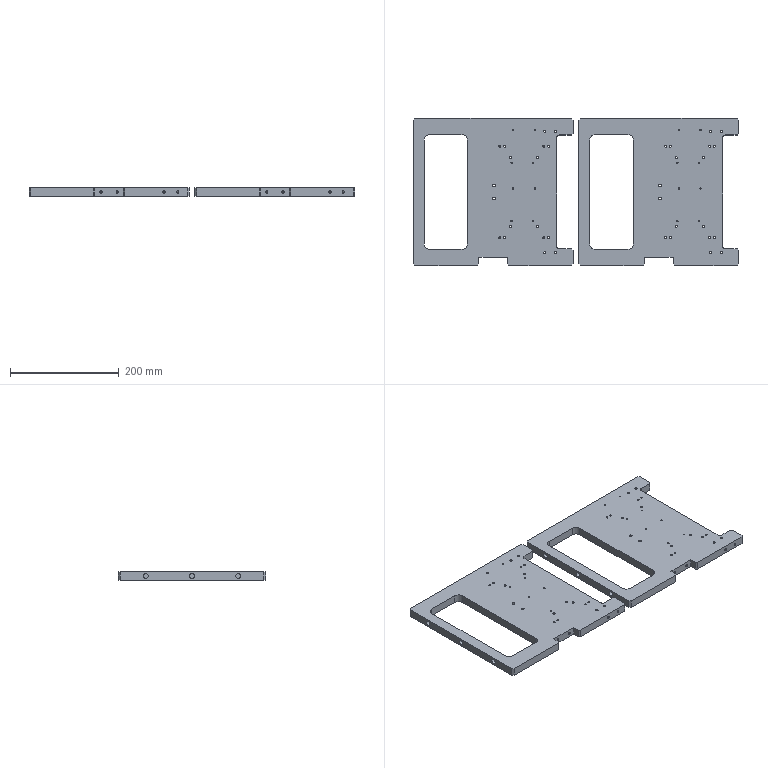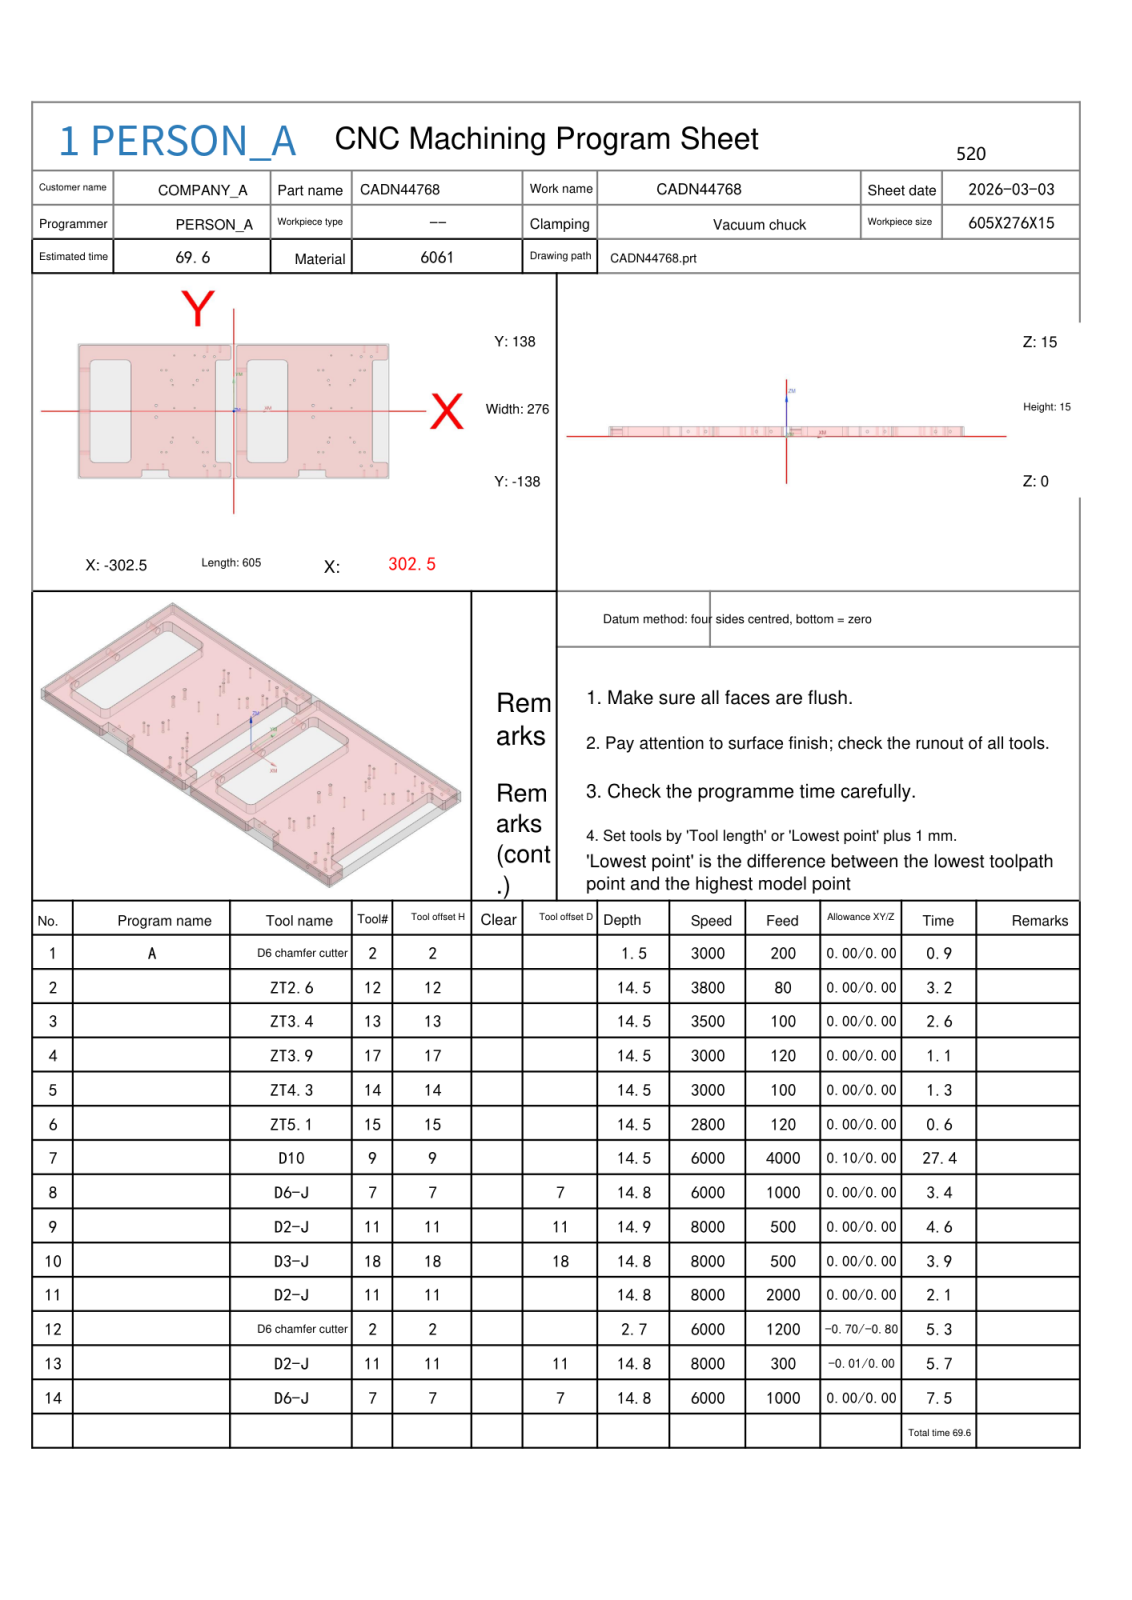NC program | NX | posted by the shop | part box 600 x 271 x 15 mm
Lines 206 to 1067 of 17346:
N7 T09 M06
(D10  D=10. R=0. H=09 ce=0.10 di=0.00)
(MAX_Z=45. MIN_Z=0.5 Time=27.42M)
G00 G90 G54 X100.4 Y0.0 M03 S6000
G43 H09 Z45.
M08
Z15.5
G01 Y95.5 Z15.41 F4000.
G03 X95.5 Y100.4 Z15.403 I-4.9 J0.0
G01 X35.5 Z15.347
G03 X30.6 Y95.5 Z15.34 I0.0 J-4.9
G01 Y-95.5 Z15.16
G03 X35.5 Y-100.4 Z15.153 I4.9 J0.0
G01 X95.5 Z15.097
G03 X100.4 Y-95.5 Z15.09 I0.0 J4.9
G01 Y95.5 Z14.91
G03 X95.5 Y100.4 Z14.903 I-4.9 J0.0
G01 X35.5 Z14.847
G03 X30.6 Y95.5 Z14.84 I0.0 J-4.9
G01 Y-95.5 Z14.66
G03 X35.5 Y-100.4 Z14.653 I4.9 J0.0
G01 X95.5 Z14.597
G03 X100.4 Y-95.5 Z14.59 I0.0 J4.9
G01 Y95.5 Z14.41
G03 X95.5 Y100.4 Z14.403 I-4.9 J0.0
G01 X35.5 Z14.347
G03 X30.6 Y95.5 Z14.34 I0.0 J-4.9
G01 Y-95.5 Z14.16
G03 X35.5 Y-100.4 Z14.153 I4.9 J0.0
G01 X95.5 Z14.097
G03 X100.4 Y-95.5 Z14.09 I0.0 J4.9
G01 Y95.5 Z13.91
G03 X95.5 Y100.4 Z13.903 I-4.9 J0.0
G01 X35.5 Z13.847
G03 X30.6 Y95.5 Z13.84 I0.0 J-4.9
G01 Y-95.5 Z13.66
G03 X35.5 Y-100.4 Z13.653 I4.9 J0.0
G01 X95.5 Z13.597
G03 X100.4 Y-95.5 Z13.59 I0.0 J4.9
G01 Y95.5 Z13.41
G03 X95.5 Y100.4 Z13.403 I-4.9 J0.0
G01 X35.5 Z13.347
G03 X30.6 Y95.5 Z13.34 I0.0 J-4.9
G01 Y-95.5 Z13.16
G03 X35.5 Y-100.4 Z13.153 I4.9 J0.0
G01 X95.5 Z13.097
G03 X100.4 Y-95.5 Z13.09 I0.0 J4.9
G01 Y95.5 Z12.91
G03 X95.5 Y100.4 Z12.903 I-4.9 J0.0
G01 X35.5 Z12.847
G03 X30.6 Y95.5 Z12.84 I0.0 J-4.9
G01 Y-95.5 Z12.66
G03 X35.5 Y-100.4 Z12.653 I4.9 J0.0
G01 X95.5 Z12.597
G03 X100.4 Y-95.5 Z12.59 I0.0 J4.9
G01 Y95.5 Z12.41
G03 X95.5 Y100.4 Z12.403 I-4.9 J0.0
G01 X35.5 Z12.347
G03 X30.6 Y95.5 Z12.34 I0.0 J-4.9
G01 Y-95.5 Z12.16
G03 X35.5 Y-100.4 Z12.153 I4.9 J0.0
G01 X95.5 Z12.097
G03 X100.4 Y-95.5 Z12.09 I0.0 J4.9
G01 Y95.5 Z11.91
G03 X95.5 Y100.4 Z11.903 I-4.9 J0.0
G01 X35.5 Z11.847
G03 X30.6 Y95.5 Z11.84 I0.0 J-4.9
G01 Y-95.5 Z11.66
G03 X35.5 Y-100.4 Z11.653 I4.9 J0.0
G01 X95.5 Z11.597
G03 X100.4 Y-95.5 Z11.59 I0.0 J4.9
G01 Y95.5 Z11.41
G03 X95.5 Y100.4 Z11.403 I-4.9 J0.0
G01 X35.5 Z11.347
G03 X30.6 Y95.5 Z11.34 I0.0 J-4.9
G01 Y-95.5 Z11.16
G03 X35.5 Y-100.4 Z11.153 I4.9 J0.0
G01 X95.5 Z11.097
G03 X100.4 Y-95.5 Z11.09 I0.0 J4.9
G01 Y95.5 Z10.91
G03 X95.5 Y100.4 Z10.903 I-4.9 J0.0
G01 X35.5 Z10.847
G03 X30.6 Y95.5 Z10.84 I0.0 J-4.9
G01 Y-95.5 Z10.66
G03 X35.5 Y-100.4 Z10.653 I4.9 J0.0
G01 X95.5 Z10.597
G03 X100.4 Y-95.5 Z10.59 I0.0 J4.9
G01 Y95.5 Z10.41
G03 X95.5 Y100.4 Z10.403 I-4.9 J0.0
G01 X35.5 Z10.347
G03 X30.6 Y95.5 Z10.34 I0.0 J-4.9
G01 Y-95.5 Z10.16
G03 X35.5 Y-100.4 Z10.153 I4.9 J0.0
G01 X95.5 Z10.097
G03 X100.4 Y-95.5 Z10.09 I0.0 J4.9
G01 Y95.5 Z9.91
G03 X95.5 Y100.4 Z9.903 I-4.9 J0.0
G01 X35.5 Z9.847
G03 X30.6 Y95.5 Z9.84 I0.0 J-4.9
G01 Y-95.5 Z9.66
G03 X35.5 Y-100.4 Z9.653 I4.9 J0.0
G01 X95.5 Z9.597
G03 X100.4 Y-95.5 Z9.59 I0.0 J4.9
G01 Y95.5 Z9.41
G03 X95.5 Y100.4 Z9.403 I-4.9 J0.0
G01 X35.5 Z9.347
G03 X30.6 Y95.5 Z9.34 I0.0 J-4.9
G01 Y-95.5 Z9.16
G03 X35.5 Y-100.4 Z9.153 I4.9 J0.0
G01 X95.5 Z9.097
G03 X100.4 Y-95.5 Z9.09 I0.0 J4.9
G01 Y95.5 Z8.91
G03 X95.5 Y100.4 Z8.903 I-4.9 J0.0
G01 X35.5 Z8.847
G03 X30.6 Y95.5 Z8.84 I0.0 J-4.9
G01 Y-95.5 Z8.66
G03 X35.5 Y-100.4 Z8.653 I4.9 J0.0
G01 X95.5 Z8.597
G03 X100.4 Y-95.5 Z8.59 I0.0 J4.9
G01 Y95.5 Z8.41
G03 X95.5 Y100.4 Z8.403 I-4.9 J0.0
G01 X35.5 Z8.347
G03 X30.6 Y95.5 Z8.34 I0.0 J-4.9
G01 Y-95.5 Z8.16
G03 X35.5 Y-100.4 Z8.153 I4.9 J0.0
G01 X95.5 Z8.097
G03 X100.4 Y-95.5 Z8.09 I0.0 J4.9
G01 Y95.5 Z7.91
G03 X95.5 Y100.4 Z7.903 I-4.9 J0.0
G01 X35.5 Z7.847
G03 X30.6 Y95.5 Z7.84 I0.0 J-4.9
G01 Y-95.5 Z7.66
G03 X35.5 Y-100.4 Z7.653 I4.9 J0.0
G01 X95.5 Z7.597
G03 X100.4 Y-95.5 Z7.59 I0.0 J4.9
G01 Y95.5 Z7.41
G03 X95.5 Y100.4 Z7.403 I-4.9 J0.0
G01 X35.5 Z7.347
G03 X30.6 Y95.5 Z7.34 I0.0 J-4.9
G01 Y-95.5 Z7.16
G03 X35.5 Y-100.4 Z7.153 I4.9 J0.0
G01 X95.5 Z7.097
G03 X100.4 Y-95.5 Z7.09 I0.0 J4.9
G01 Y95.5 Z6.91
G03 X95.5 Y100.4 Z6.903 I-4.9 J0.0
G01 X35.5 Z6.847
G03 X30.6 Y95.5 Z6.84 I0.0 J-4.9
G01 Y-95.5 Z6.66
G03 X35.5 Y-100.4 Z6.653 I4.9 J0.0
G01 X95.5 Z6.597
G03 X100.4 Y-95.5 Z6.59 I0.0 J4.9
G01 Y95.5 Z6.41
G03 X95.5 Y100.4 Z6.403 I-4.9 J0.0
G01 X35.5 Z6.347
G03 X30.6 Y95.5 Z6.34 I0.0 J-4.9
G01 Y-95.5 Z6.16
G03 X35.5 Y-100.4 Z6.153 I4.9 J0.0
G01 X95.5 Z6.097
G03 X100.4 Y-95.5 Z6.09 I0.0 J4.9
G01 Y95.5 Z5.91
G03 X95.5 Y100.4 Z5.903 I-4.9 J0.0
G01 X35.5 Z5.847
G03 X30.6 Y95.5 Z5.84 I0.0 J-4.9
G01 Y-95.5 Z5.66
G03 X35.5 Y-100.4 Z5.653 I4.9 J0.0
G01 X95.5 Z5.597
G03 X100.4 Y-95.5 Z5.59 I0.0 J4.9
G01 Y95.5 Z5.41
G03 X95.5 Y100.4 Z5.403 I-4.9 J0.0
G01 X35.5 Z5.347
G03 X30.6 Y95.5 Z5.34 I0.0 J-4.9
G01 Y-95.5 Z5.16
G03 X35.5 Y-100.4 Z5.153 I4.9 J0.0
G01 X95.5 Z5.097
G03 X100.4 Y-95.5 Z5.09 I0.0 J4.9
G01 Y95.5 Z4.91
G03 X95.5 Y100.4 Z4.903 I-4.9 J0.0
G01 X35.5 Z4.847
G03 X30.6 Y95.5 Z4.84 I0.0 J-4.9
G01 Y-95.5 Z4.66
G03 X35.5 Y-100.4 Z4.653 I4.9 J0.0
G01 X95.5 Z4.597
G03 X100.4 Y-95.5 Z4.59 I0.0 J4.9
G01 Y95.5 Z4.41
G03 X95.5 Y100.4 Z4.403 I-4.9 J0.0
G01 X35.5 Z4.347
G03 X30.6 Y95.5 Z4.34 I0.0 J-4.9
G01 Y-95.5 Z4.16
G03 X35.5 Y-100.4 Z4.153 I4.9 J0.0
G01 X95.5 Z4.097
G03 X100.4 Y-95.5 Z4.09 I0.0 J4.9
G01 Y95.5 Z3.91
G03 X95.5 Y100.4 Z3.903 I-4.9 J0.0
G01 X35.5 Z3.847
G03 X30.6 Y95.5 Z3.84 I0.0 J-4.9
G01 Y-95.5 Z3.66
G03 X35.5 Y-100.4 Z3.653 I4.9 J0.0
G01 X95.5 Z3.597
G03 X100.4 Y-95.5 Z3.59 I0.0 J4.9
G01 Y95.5 Z3.41
G03 X95.5 Y100.4 Z3.403 I-4.9 J0.0
G01 X35.5 Z3.347
G03 X30.6 Y95.5 Z3.34 I0.0 J-4.9
G01 Y-95.5 Z3.16
G03 X35.5 Y-100.4 Z3.153 I4.9 J0.0
G01 X95.5 Z3.097
G03 X100.4 Y-95.5 Z3.09 I0.0 J4.9
G01 Y95.5 Z2.91
G03 X95.5 Y100.4 Z2.903 I-4.9 J0.0
G01 X35.5 Z2.847
G03 X30.6 Y95.5 Z2.84 I0.0 J-4.9
G01 Y-95.5 Z2.66
G03 X35.5 Y-100.4 Z2.653 I4.9 J0.0
G01 X95.5 Z2.597
G03 X100.4 Y-95.5 Z2.59 I0.0 J4.9
G01 Y95.5 Z2.41
G03 X95.5 Y100.4 Z2.403 I-4.9 J0.0
G01 X35.5 Z2.347
G03 X30.6 Y95.5 Z2.34 I0.0 J-4.9
G01 Y-95.5 Z2.16
G03 X35.5 Y-100.4 Z2.153 I4.9 J0.0
G01 X95.5 Z2.097
G03 X100.4 Y-95.5 Z2.09 I0.0 J4.9
G01 Y95.5 Z1.91
G03 X95.5 Y100.4 Z1.903 I-4.9 J0.0
G01 X35.5 Z1.847
G03 X30.6 Y95.5 Z1.84 I0.0 J-4.9
G01 Y-95.5 Z1.66
G03 X35.5 Y-100.4 Z1.653 I4.9 J0.0
G01 X95.5 Z1.597
G03 X100.4 Y-95.5 Z1.59 I0.0 J4.9
G01 Y95.5 Z1.41
G03 X95.5 Y100.4 Z1.403 I-4.9 J0.0
G01 X35.5 Z1.347
G03 X30.6 Y95.5 Z1.34 I0.0 J-4.9
G01 Y-95.5 Z1.16
G03 X35.5 Y-100.4 Z1.153 I4.9 J0.0
G01 X95.5 Z1.097
G03 X100.4 Y-95.5 Z1.09 I0.0 J4.9
G01 Y95.5 Z.91
G03 X95.5 Y100.4 Z.903 I-4.9 J0.0
G01 X35.5 Z.847
G03 X30.6 Y95.5 Z.84 I0.0 J-4.9
G01 Y-95.5 Z.66
G03 X35.5 Y-100.4 Z.653 I4.9 J0.0
G01 X95.5 Z.597
G03 X100.4 Y-95.5 Z.59 I0.0 J4.9
G01 Y0.0 Z.5
Y95.5
G03 X95.5 Y100.4 I-4.9 J0.0
G01 X35.5
G03 X30.6 Y95.5 I0.0 J-4.9
G01 Y-95.5
G03 X35.5 Y-100.4 I4.9 J0.0
G01 X95.5
G03 X100.4 Y-95.5 I0.0 J4.9
G01 Y0.0
Y.5
Z1.5
G00 Z45.
X-274.9 Y0.0
Z15.5
G01 Y-95.5 Z15.41
G03 X-270. Y-100.4 Z15.403 I4.9 J0.0
G01 X-210. Z15.347
G03 X-205.1 Y-95.5 Z15.34 I0.0 J4.9
G01 Y95.5 Z15.16
G03 X-210. Y100.4 Z15.153 I-4.9 J0.0
G01 X-270. Z15.097
G03 X-274.9 Y95.5 Z15.09 I0.0 J-4.9
G01 Y-95.5 Z14.91
G03 X-270. Y-100.4 Z14.903 I4.9 J0.0
G01 X-210. Z14.847
G03 X-205.1 Y-95.5 Z14.84 I0.0 J4.9
G01 Y95.5 Z14.66
G03 X-210. Y100.4 Z14.653 I-4.9 J0.0
G01 X-270. Z14.597
G03 X-274.9 Y95.5 Z14.59 I0.0 J-4.9
G01 Y-95.5 Z14.41
G03 X-270. Y-100.4 Z14.403 I4.9 J0.0
G01 X-210. Z14.347
G03 X-205.1 Y-95.5 Z14.34 I0.0 J4.9
G01 Y95.5 Z14.16
G03 X-210. Y100.4 Z14.153 I-4.9 J0.0
G01 X-270. Z14.097
G03 X-274.9 Y95.5 Z14.09 I0.0 J-4.9
G01 Y-95.5 Z13.91
G03 X-270. Y-100.4 Z13.903 I4.9 J0.0
G01 X-210. Z13.847
G03 X-205.1 Y-95.5 Z13.84 I0.0 J4.9
G01 Y95.5 Z13.66
G03 X-210. Y100.4 Z13.653 I-4.9 J0.0
G01 X-270. Z13.597
G03 X-274.9 Y95.5 Z13.59 I0.0 J-4.9
G01 Y-95.5 Z13.41
G03 X-270. Y-100.4 Z13.403 I4.9 J0.0
G01 X-210. Z13.347
G03 X-205.1 Y-95.5 Z13.34 I0.0 J4.9
G01 Y95.5 Z13.16
G03 X-210. Y100.4 Z13.153 I-4.9 J0.0
G01 X-270. Z13.097
G03 X-274.9 Y95.5 Z13.09 I0.0 J-4.9
G01 Y-95.5 Z12.91
G03 X-270. Y-100.4 Z12.903 I4.9 J0.0
G01 X-210. Z12.847
G03 X-205.1 Y-95.5 Z12.84 I0.0 J4.9
G01 Y95.5 Z12.66
G03 X-210. Y100.4 Z12.653 I-4.9 J0.0
G01 X-270. Z12.597
G03 X-274.9 Y95.5 Z12.59 I0.0 J-4.9
G01 Y-95.5 Z12.41
G03 X-270. Y-100.4 Z12.403 I4.9 J0.0
G01 X-210. Z12.347
G03 X-205.1 Y-95.5 Z12.34 I0.0 J4.9
G01 Y95.5 Z12.16
G03 X-210. Y100.4 Z12.153 I-4.9 J0.0
G01 X-270. Z12.097
G03 X-274.9 Y95.5 Z12.09 I0.0 J-4.9
G01 Y-95.5 Z11.91
G03 X-270. Y-100.4 Z11.903 I4.9 J0.0
G01 X-210. Z11.847
G03 X-205.1 Y-95.5 Z11.84 I0.0 J4.9
G01 Y95.5 Z11.66
G03 X-210. Y100.4 Z11.653 I-4.9 J0.0
G01 X-270. Z11.597
G03 X-274.9 Y95.5 Z11.59 I0.0 J-4.9
G01 Y-95.5 Z11.41
G03 X-270. Y-100.4 Z11.403 I4.9 J0.0
G01 X-210. Z11.347
G03 X-205.1 Y-95.5 Z11.34 I0.0 J4.9
G01 Y95.5 Z11.16
G03 X-210. Y100.4 Z11.153 I-4.9 J0.0
G01 X-270. Z11.097
G03 X-274.9 Y95.5 Z11.09 I0.0 J-4.9
G01 Y-95.5 Z10.91
G03 X-270. Y-100.4 Z10.903 I4.9 J0.0
G01 X-210. Z10.847
G03 X-205.1 Y-95.5 Z10.84 I0.0 J4.9
G01 Y95.5 Z10.66
G03 X-210. Y100.4 Z10.653 I-4.9 J0.0
G01 X-270. Z10.597
G03 X-274.9 Y95.5 Z10.59 I0.0 J-4.9
G01 Y-95.5 Z10.41
G03 X-270. Y-100.4 Z10.403 I4.9 J0.0
G01 X-210. Z10.347
G03 X-205.1 Y-95.5 Z10.34 I0.0 J4.9
G01 Y95.5 Z10.16
G03 X-210. Y100.4 Z10.153 I-4.9 J0.0
G01 X-270. Z10.097
G03 X-274.9 Y95.5 Z10.09 I0.0 J-4.9
G01 Y-95.5 Z9.91
G03 X-270. Y-100.4 Z9.903 I4.9 J0.0
G01 X-210. Z9.847
G03 X-205.1 Y-95.5 Z9.84 I0.0 J4.9
G01 Y95.5 Z9.66
G03 X-210. Y100.4 Z9.653 I-4.9 J0.0
G01 X-270. Z9.597
G03 X-274.9 Y95.5 Z9.59 I0.0 J-4.9
G01 Y-95.5 Z9.41
G03 X-270. Y-100.4 Z9.403 I4.9 J0.0
G01 X-210. Z9.347
G03 X-205.1 Y-95.5 Z9.34 I0.0 J4.9
G01 Y95.5 Z9.16
G03 X-210. Y100.4 Z9.153 I-4.9 J0.0
G01 X-270. Z9.097
G03 X-274.9 Y95.5 Z9.09 I0.0 J-4.9
G01 Y-95.5 Z8.91
G03 X-270. Y-100.4 Z8.903 I4.9 J0.0
G01 X-210. Z8.847
G03 X-205.1 Y-95.5 Z8.84 I0.0 J4.9
G01 Y95.5 Z8.66
G03 X-210. Y100.4 Z8.653 I-4.9 J0.0
G01 X-270. Z8.597
G03 X-274.9 Y95.5 Z8.59 I0.0 J-4.9
G01 Y-95.5 Z8.41
G03 X-270. Y-100.4 Z8.403 I4.9 J0.0
G01 X-210. Z8.347
G03 X-205.1 Y-95.5 Z8.34 I0.0 J4.9
G01 Y95.5 Z8.16
G03 X-210. Y100.4 Z8.153 I-4.9 J0.0
G01 X-270. Z8.097
G03 X-274.9 Y95.5 Z8.09 I0.0 J-4.9
G01 Y-95.5 Z7.91
G03 X-270. Y-100.4 Z7.903 I4.9 J0.0
G01 X-210. Z7.847
G03 X-205.1 Y-95.5 Z7.84 I0.0 J4.9
G01 Y95.5 Z7.66
G03 X-210. Y100.4 Z7.653 I-4.9 J0.0
G01 X-270. Z7.597
G03 X-274.9 Y95.5 Z7.59 I0.0 J-4.9
G01 Y-95.5 Z7.41
G03 X-270. Y-100.4 Z7.403 I4.9 J0.0
G01 X-210. Z7.347
G03 X-205.1 Y-95.5 Z7.34 I0.0 J4.9
G01 Y95.5 Z7.16
G03 X-210. Y100.4 Z7.153 I-4.9 J0.0
G01 X-270. Z7.097
G03 X-274.9 Y95.5 Z7.09 I0.0 J-4.9
G01 Y-95.5 Z6.91
G03 X-270. Y-100.4 Z6.903 I4.9 J0.0
G01 X-210. Z6.847
G03 X-205.1 Y-95.5 Z6.84 I0.0 J4.9
G01 Y95.5 Z6.66
G03 X-210. Y100.4 Z6.653 I-4.9 J0.0
G01 X-270. Z6.597
G03 X-274.9 Y95.5 Z6.59 I0.0 J-4.9
G01 Y-95.5 Z6.41
G03 X-270. Y-100.4 Z6.403 I4.9 J0.0
G01 X-210. Z6.347
G03 X-205.1 Y-95.5 Z6.34 I0.0 J4.9
G01 Y95.5 Z6.16
G03 X-210. Y100.4 Z6.153 I-4.9 J0.0
G01 X-270. Z6.097
G03 X-274.9 Y95.5 Z6.09 I0.0 J-4.9
G01 Y-95.5 Z5.91
G03 X-270. Y-100.4 Z5.903 I4.9 J0.0
G01 X-210. Z5.847
G03 X-205.1 Y-95.5 Z5.84 I0.0 J4.9
G01 Y95.5 Z5.66
G03 X-210. Y100.4 Z5.653 I-4.9 J0.0
G01 X-270. Z5.597
G03 X-274.9 Y95.5 Z5.59 I0.0 J-4.9
G01 Y-95.5 Z5.41
G03 X-270. Y-100.4 Z5.403 I4.9 J0.0
G01 X-210. Z5.347
G03 X-205.1 Y-95.5 Z5.34 I0.0 J4.9
G01 Y95.5 Z5.16
G03 X-210. Y100.4 Z5.153 I-4.9 J0.0
G01 X-270. Z5.097
G03 X-274.9 Y95.5 Z5.09 I0.0 J-4.9
G01 Y-95.5 Z4.91
G03 X-270. Y-100.4 Z4.903 I4.9 J0.0
G01 X-210. Z4.847
G03 X-205.1 Y-95.5 Z4.84 I0.0 J4.9
G01 Y95.5 Z4.66
G03 X-210. Y100.4 Z4.653 I-4.9 J0.0
G01 X-270. Z4.597
G03 X-274.9 Y95.5 Z4.59 I0.0 J-4.9
G01 Y-95.5 Z4.41
G03 X-270. Y-100.4 Z4.403 I4.9 J0.0
G01 X-210. Z4.347
G03 X-205.1 Y-95.5 Z4.34 I0.0 J4.9
G01 Y95.5 Z4.16
G03 X-210. Y100.4 Z4.153 I-4.9 J0.0
G01 X-270. Z4.097
G03 X-274.9 Y95.5 Z4.09 I0.0 J-4.9
G01 Y-95.5 Z3.91
G03 X-270. Y-100.4 Z3.903 I4.9 J0.0
G01 X-210. Z3.847
G03 X-205.1 Y-95.5 Z3.84 I0.0 J4.9
G01 Y95.5 Z3.66
G03 X-210. Y100.4 Z3.653 I-4.9 J0.0
G01 X-270. Z3.597
G03 X-274.9 Y95.5 Z3.59 I0.0 J-4.9
G01 Y-95.5 Z3.41
G03 X-270. Y-100.4 Z3.403 I4.9 J0.0
G01 X-210. Z3.347
G03 X-205.1 Y-95.5 Z3.34 I0.0 J4.9
G01 Y95.5 Z3.16
G03 X-210. Y100.4 Z3.153 I-4.9 J0.0
G01 X-270. Z3.097
G03 X-274.9 Y95.5 Z3.09 I0.0 J-4.9
G01 Y-95.5 Z2.91
G03 X-270. Y-100.4 Z2.903 I4.9 J0.0
G01 X-210. Z2.847
G03 X-205.1 Y-95.5 Z2.84 I0.0 J4.9
G01 Y95.5 Z2.66
G03 X-210. Y100.4 Z2.653 I-4.9 J0.0
G01 X-270. Z2.597
G03 X-274.9 Y95.5 Z2.59 I0.0 J-4.9
G01 Y-95.5 Z2.41
G03 X-270. Y-100.4 Z2.403 I4.9 J0.0
G01 X-210. Z2.347
G03 X-205.1 Y-95.5 Z2.34 I0.0 J4.9
G01 Y95.5 Z2.16
G03 X-210. Y100.4 Z2.153 I-4.9 J0.0
G01 X-270. Z2.097
G03 X-274.9 Y95.5 Z2.09 I0.0 J-4.9
G01 Y-95.5 Z1.91
G03 X-270. Y-100.4 Z1.903 I4.9 J0.0
G01 X-210. Z1.847
G03 X-205.1 Y-95.5 Z1.84 I0.0 J4.9
G01 Y95.5 Z1.66
G03 X-210. Y100.4 Z1.653 I-4.9 J0.0
G01 X-270. Z1.597
G03 X-274.9 Y95.5 Z1.59 I0.0 J-4.9
G01 Y-95.5 Z1.41
G03 X-270. Y-100.4 Z1.403 I4.9 J0.0
G01 X-210. Z1.347
G03 X-205.1 Y-95.5 Z1.34 I0.0 J4.9
G01 Y95.5 Z1.16
G03 X-210. Y100.4 Z1.153 I-4.9 J0.0
G01 X-270. Z1.097
G03 X-274.9 Y95.5 Z1.09 I0.0 J-4.9
G01 Y-95.5 Z.91
G03 X-270. Y-100.4 Z.903 I4.9 J0.0
G01 X-210. Z.847
G03 X-205.1 Y-95.5 Z.84 I0.0 J4.9
G01 Y95.5 Z.66
G03 X-210. Y100.4 Z.653 I-4.9 J0.0
G01 X-270. Z.597
G03 X-274.9 Y95.5 Z.59 I0.0 J-4.9
G01 Y0.0 Z.5
Y-95.5
G03 X-270. Y-100.4 I4.9 J0.0
G01 X-210.
G03 X-205.1 Y-95.5 I0.0 J4.9
G01 Y95.5
G03 X-210. Y100.4 I-4.9 J0.0
G01 X-270.
G03 X-274.9 Y95.5 I0.0 J-4.9
G01 Y0.0
Y-.5
Z1.5
G00 Z45.
G00 G90 X-152.75 Y140.6 M03 S6000
Z45.
Z15.5
G01 X-8.5 Z15.441 F4000.
G02 X-4.894 Y139.106 Z15.44 I0.0 J-5.1
G01 X-1.894 Y136.106 Z15.438
G02 X-.4 Y132.5 Z15.436 I-3.606 J-3.606
G01 Y108. Z15.426
G02 X-1.894 Y104.394 Z15.425 I-5.1 J0.0
G01 X-4.894 Y101.394 Z15.423
G02 X-8.5 Y99.9 Z15.421 I-3.606 J3.606
G01 X-30.4 Z15.413
Y-99.9 Z15.331
X-8.5 Z15.322
G02 X-4.894 Y-101.394 Z15.321 I0.0 J-5.1
G01 X-1.894 Y-104.394 Z15.319
G02 X-.4 Y-108. Z15.317 I-3.606 J-3.606
G01 Y-132.5 Z15.308
G02 X-1.894 Y-136.106 Z15.306 I-5.1 J0.0
G01 X-4.894 Y-139.106 Z15.304
G02 X-8.5 Y-140.6 Z15.303 I-3.606 J3.606
G01 X-123.75 Z15.256
G02 X-127.356 Y-139.106 Z15.254 I0.0 J5.1
G01 X-130.356 Y-136.106 Z15.252
G02 X-131.85 Y-132.5 Z15.251 I3.606 J3.606
G01 Y-125.6 Z15.248
X-173.65 Z15.231
Y-132.5 Z15.228
G02 X-175.144 Y-136.106 Z15.226 I-5.1 J0.0
G01 X-178.144 Y-139.106 Z15.225
G02 X-181.75 Y-140.6 Z15.223 I-3.606 J3.606
G01 X-297. Z15.176
G02 X-300.606 Y-139.106 Z15.175 I0.0 J5.1
G01 X-303.606 Y-136.106 Z15.173
G02 X-305.1 Y-132.5 Z15.171 I3.606 J3.606
G01 Y132.5 Z15.064
G02 X-303.606 Y136.106 Z15.062 I5.1 J0.0
G01 X-300.606 Y139.106 Z15.06
G02 X-298.786 Y140.277 Z15.059 I3.606 J-3.606
X-297. Y140.6 Z15.059 I1.786 J-4.777
G01 X-8.5 Z14.941
G02 X-4.894 Y139.106 Z14.94 I0.0 J-5.1
G01 X-1.894 Y136.106 Z14.938
G02 X-.4 Y132.5 Z14.936 I-3.606 J-3.606
G01 Y108. Z14.926
G02 X-1.894 Y104.394 Z14.925 I-5.1 J0.0
G01 X-4.894 Y101.394 Z14.923
G02 X-8.5 Y99.9 Z14.921 I-3.606 J3.606
G01 X-30.4 Z14.913
Y-99.9 Z14.831
X-8.5 Z14.822
G02 X-4.894 Y-101.394 Z14.821 I0.0 J-5.1
G01 X-1.894 Y-104.394 Z14.819
G02 X-.4 Y-108. Z14.817 I-3.606 J-3.606
G01 Y-132.5 Z14.808
G02 X-1.894 Y-136.106 Z14.806 I-5.1 J0.0
G01 X-4.894 Y-139.106 Z14.804
G02 X-8.5 Y-140.6 Z14.803 I-3.606 J3.606
G01 X-123.75 Z14.756
G02 X-127.356 Y-139.106 Z14.754 I0.0 J5.1
G01 X-130.356 Y-136.106 Z14.752
G02 X-131.85 Y-132.5 Z14.751 I3.606 J3.606
G01 Y-125.6 Z14.748
X-173.65 Z14.731
Y-132.5 Z14.728
G02 X-175.144 Y-136.106 Z14.726 I-5.1 J0.0
G01 X-178.144 Y-139.106 Z14.725
G02 X-181.75 Y-140.6 Z14.723 I-3.606 J3.606
G01 X-297. Z14.676
G02 X-300.606 Y-139.106 Z14.675 I0.0 J5.1
G01 X-303.606 Y-136.106 Z14.673
G02 X-305.1 Y-132.5 Z14.671 I3.606 J3.606
G01 Y132.5 Z14.564
G02 X-303.606 Y136.106 Z14.562 I5.1 J0.0
G01 X-300.606 Y139.106 Z14.56
G02 X-298.786 Y140.277 Z14.559 I3.606 J-3.606
X-297. Y140.6 Z14.559 I1.786 J-4.777
G01 X-8.5 Z14.441
G02 X-4.894 Y139.106 Z14.44 I0.0 J-5.1
G01 X-1.894 Y136.106 Z14.438
G02 X-.4 Y132.5 Z14.436 I-3.606 J-3.606
G01 Y108. Z14.426
G02 X-1.894 Y104.394 Z14.425 I-5.1 J0.0
G01 X-4.894 Y101.394 Z14.423
G02 X-8.5 Y99.9 Z14.421 I-3.606 J3.606
G01 X-30.4 Z14.413
Y-99.9 Z14.331
X-8.5 Z14.322
G02 X-4.894 Y-101.394 Z14.321 I0.0 J-5.1
G01 X-1.894 Y-104.394 Z14.319
G02 X-.4 Y-108. Z14.317 I-3.606 J-3.606
G01 Y-132.5 Z14.308
G02 X-1.894 Y-136.106 Z14.306 I-5.1 J0.0
G01 X-4.894 Y-139.106 Z14.304
G02 X-8.5 Y-140.6 Z14.303 I-3.606 J3.606
G01 X-123.75 Z14.256
G02 X-127.356 Y-139.106 Z14.254 I0.0 J5.1
G01 X-130.356 Y-136.106 Z14.252
G02 X-131.85 Y-132.5 Z14.251 I3.606 J3.606
G01 Y-125.6 Z14.248
X-173.65 Z14.231
Y-132.5 Z14.228
G02 X-175.144 Y-136.106 Z14.226 I-5.1 J0.0
G01 X-178.144 Y-139.106 Z14.225
G02 X-181.75 Y-140.6 Z14.223 I-3.606 J3.606
G01 X-297. Z14.176
G02 X-300.606 Y-139.106 Z14.175 I0.0 J5.1
G01 X-303.606 Y-136.106 Z14.173
G02 X-305.1 Y-132.5 Z14.171 I3.606 J3.606
G01 Y132.5 Z14.064
G02 X-303.606 Y136.106 Z14.062 I5.1 J0.0
G01 X-300.606 Y139.106 Z14.06
G02 X-298.786 Y140.277 Z14.059 I3.606 J-3.606
X-297. Y140.6 Z14.059 I1.786 J-4.777
G01 X-8.5 Z13.941
G02 X-4.894 Y139.106 Z13.94 I0.0 J-5.1
G01 X-1.894 Y136.106 Z13.938
G02 X-.4 Y132.5 Z13.936 I-3.606 J-3.606
G01 Y108. Z13.926
G02 X-1.894 Y104.394 Z13.925 I-5.1 J0.0
G01 X-4.894 Y101.394 Z13.923
G02 X-8.5 Y99.9 Z13.921 I-3.606 J3.606
G01 X-30.4 Z13.913
Y-99.9 Z13.831
X-8.5 Z13.822
G02 X-4.894 Y-101.394 Z13.821 I0.0 J-5.1
G01 X-1.894 Y-104.394 Z13.819
G02 X-.4 Y-108. Z13.817 I-3.606 J-3.606
G01 Y-132.5 Z13.808
G02 X-1.894 Y-136.106 Z13.806 I-5.1 J0.0
G01 X-4.894 Y-139.106 Z13.804
G02 X-8.5 Y-140.6 Z13.803 I-3.606 J3.606
G01 X-123.75 Z13.756
G02 X-127.356 Y-139.106 Z13.754 I0.0 J5.1
G01 X-130.356 Y-136.106 Z13.752
G02 X-131.85 Y-132.5 Z13.751 I3.606 J3.606
G01 Y-125.6 Z13.748
X-173.65 Z13.731
Y-132.5 Z13.728
G02 X-175.144 Y-136.106 Z13.726 I-5.1 J0.0
G01 X-178.144 Y-139.106 Z13.725
G02 X-181.75 Y-140.6 Z13.723 I-3.606 J3.606
G01 X-297. Z13.676
G02 X-300.606 Y-139.106 Z13.675 I0.0 J5.1
G01 X-303.606 Y-136.106 Z13.673
G02 X-305.1 Y-132.5 Z13.671 I3.606 J3.606
G01 Y132.5 Z13.564
G02 X-303.606 Y136.106 Z13.562 I5.1 J0.0
G01 X-300.606 Y139.106 Z13.56
G02 X-298.786 Y140.277 Z13.559 I3.606 J-3.606
X-297. Y140.6 Z13.559 I1.786 J-4.777
G01 X-8.5 Z13.441
G02 X-4.894 Y139.106 Z13.44 I0.0 J-5.1
G01 X-1.894 Y136.106 Z13.438
G02 X-.4 Y132.5 Z13.436 I-3.606 J-3.606
G01 Y108. Z13.426
G02 X-1.894 Y104.394 Z13.425 I-5.1 J0.0
G01 X-4.894 Y101.394 Z13.423
G02 X-8.5 Y99.9 Z13.421 I-3.606 J3.606
G01 X-30.4 Z13.413
Y-99.9 Z13.331
X-8.5 Z13.322
G02 X-4.894 Y-101.394 Z13.321 I0.0 J-5.1
G01 X-1.894 Y-104.394 Z13.319
G02 X-.4 Y-108. Z13.317 I-3.606 J-3.606
G01 Y-132.5 Z13.308
G02 X-1.894 Y-136.106 Z13.306 I-5.1 J0.0
G01 X-4.894 Y-139.106 Z13.304
G02 X-8.5 Y-140.6 Z13.303 I-3.606 J3.606
G01 X-123.75 Z13.256
G02 X-127.356 Y-139.106 Z13.254 I0.0 J5.1
G01 X-130.356 Y-136.106 Z13.252
G02 X-131.85 Y-132.5 Z13.251 I3.606 J3.606
G01 Y-125.6 Z13.248
X-173.65 Z13.231
Y-132.5 Z13.228
G02 X-175.144 Y-136.106 Z13.226 I-5.1 J0.0
G01 X-178.144 Y-139.106 Z13.225
G02 X-181.75 Y-140.6 Z13.223 I-3.606 J3.606
G01 X-297. Z13.176
G02 X-300.606 Y-139.106 Z13.175 I0.0 J5.1
G01 X-303.606 Y-136.106 Z13.173
G02 X-305.1 Y-132.5 Z13.171 I3.606 J3.606
G01 Y132.5 Z13.064
G02 X-303.606 Y136.106 Z13.062 I5.1 J0.0
G01 X-300.606 Y139.106 Z13.06
G02 X-298.786 Y140.277 Z13.059 I3.606 J-3.606
X-297. Y140.6 Z13.059 I1.786 J-4.777
G01 X-8.5 Z12.941
G02 X-4.894 Y139.106 Z12.94 I0.0 J-5.1
G01 X-1.894 Y136.106 Z12.938
G02 X-.4 Y132.5 Z12.936 I-3.606 J-3.606
G01 Y108. Z12.926
G02 X-1.894 Y104.394 Z12.925 I-5.1 J0.0
G01 X-4.894 Y101.394 Z12.923
G02 X-8.5 Y99.9 Z12.921 I-3.606 J3.606
G01 X-30.4 Z12.913
Y-99.9 Z12.831
X-8.5 Z12.822
G02 X-4.894 Y-101.394 Z12.821 I0.0 J-5.1
G01 X-1.894 Y-104.394 Z12.819
G02 X-.4 Y-108. Z12.817 I-3.606 J-3.606
G01 Y-132.5 Z12.808
G02 X-1.894 Y-136.106 Z12.806 I-5.1 J0.0
G01 X-4.894 Y-139.106 Z12.804
G02 X-8.5 Y-140.6 Z12.803 I-3.606 J3.606
G01 X-123.75 Z12.756
G02 X-127.356 Y-139.106 Z12.754 I0.0 J5.1
G01 X-130.356 Y-136.106 Z12.752
G02 X-131.85 Y-132.5 Z12.751 I3.606 J3.606
G01 Y-125.6 Z12.748
X-173.65 Z12.731
Y-132.5 Z12.728
G02 X-175.144 Y-136.106 Z12.726 I-5.1 J0.0
G01 X-178.144 Y-139.106 Z12.725
G02 X-181.75 Y-140.6 Z12.723 I-3.606 J3.606
G01 X-297. Z12.676
G02 X-300.606 Y-139.106 Z12.675 I0.0 J5.1
G01 X-303.606 Y-136.106 Z12.673
G02 X-305.1 Y-132.5 Z12.671 I3.606 J3.606
G01 Y132.5 Z12.564
G02 X-303.606 Y136.106 Z12.562 I5.1 J0.0
G01 X-300.606 Y139.106 Z12.56
G02 X-298.786 Y140.277 Z12.559 I3.606 J-3.606
X-297. Y140.6 Z12.559 I1.786 J-4.777
G01 X-8.5 Z12.441
G02 X-4.894 Y139.106 Z12.44 I0.0 J-5.1
G01 X-1.894 Y136.106 Z12.438
G02 X-.4 Y132.5 Z12.436 I-3.606 J-3.606
G01 Y108. Z12.426
G02 X-1.894 Y104.394 Z12.425 I-5.1 J0.0
G01 X-4.894 Y101.394 Z12.423
G02 X-8.5 Y99.9 Z12.421 I-3.606 J3.606
G01 X-30.4 Z12.413
Y-99.9 Z12.331
X-8.5 Z12.322
G02 X-4.894 Y-101.394 Z12.321 I0.0 J-5.1
G01 X-1.894 Y-104.394 Z12.319
G02 X-.4 Y-108. Z12.317 I-3.606 J-3.606
G01 Y-132.5 Z12.308
G02 X-1.894 Y-136.106 Z12.306 I-5.1 J0.0
G01 X-4.894 Y-139.106 Z12.304
G02 X-8.5 Y-140.6 Z12.303 I-3.606 J3.606
G01 X-123.75 Z12.256
G02 X-127.356 Y-139.106 Z12.254 I0.0 J5.1
G01 X-130.356 Y-136.106 Z12.252
G02 X-131.85 Y-132.5 Z12.251 I3.606 J3.606
G01 Y-125.6 Z12.248
X-173.65 Z12.231
Y-132.5 Z12.228
G02 X-175.144 Y-136.106 Z12.226 I-5.1 J0.0
G01 X-178.144 Y-139.106 Z12.225
G02 X-181.75 Y-140.6 Z12.223 I-3.606 J3.606
G01 X-297. Z12.176
G02 X-300.606 Y-139.106 Z12.175 I0.0 J5.1
G01 X-303.606 Y-136.106 Z12.173
G02 X-305.1 Y-132.5 Z12.171 I3.606 J3.606
G01 Y132.5 Z12.064
G02 X-303.606 Y136.106 Z12.062 I5.1 J0.0
G01 X-300.606 Y139.106 Z12.06
G02 X-298.786 Y140.277 Z12.059 I3.606 J-3.606
X-297. Y140.6 Z12.059 I1.786 J-4.777
G01 X-8.5 Z11.941
G02 X-4.894 Y139.106 Z11.94 I0.0 J-5.1
G01 X-1.894 Y136.106 Z11.938
G02 X-.4 Y132.5 Z11.936 I-3.606 J-3.606
G01 Y108. Z11.926
G02 X-1.894 Y104.394 Z11.925 I-5.1 J0.0
G01 X-4.894 Y101.394 Z11.923
G02 X-8.5 Y99.9 Z11.921 I-3.606 J3.606
G01 X-30.4 Z11.913
Y-99.9 Z11.831
X-8.5 Z11.822
G02 X-4.894 Y-101.394 Z11.821 I0.0 J-5.1
G01 X-1.894 Y-104.394 Z11.819
G02 X-.4 Y-108. Z11.817 I-3.606 J-3.606
G01 Y-132.5 Z11.808
G02 X-1.894 Y-136.106 Z11.806 I-5.1 J0.0
G01 X-4.894 Y-139.106 Z11.804
G02 X-8.5 Y-140.6 Z11.803 I-3.606 J3.606
G01 X-123.75 Z11.756
G02 X-127.356 Y-139.106 Z11.754 I0.0 J5.1
G01 X-130.356 Y-136.106 Z11.752
G02 X-131.85 Y-132.5 Z11.751 I3.606 J3.606
G01 Y-125.6 Z11.748
X-173.65 Z11.731
Y-132.5 Z11.728
G02 X-175.144 Y-136.106 Z11.726 I-5.1 J0.0
G01 X-178.144 Y-139.106 Z11.725
G02 X-181.75 Y-140.6 Z11.723 I-3.606 J3.606
G01 X-297. Z11.676
G02 X-300.606 Y-139.106 Z11.675 I0.0 J5.1
G01 X-303.606 Y-136.106 Z11.673
G02 X-305.1 Y-132.5 Z11.671 I3.606 J3.606
G01 Y132.5 Z11.564
G02 X-303.606 Y136.106 Z11.562 I5.1 J0.0
G01 X-300.606 Y139.106 Z11.56
G02 X-298.786 Y140.277 Z11.559 I3.606 J-3.606
X-297. Y140.6 Z11.559 I1.786 J-4.777
G01 X-8.5 Z11.441
G02 X-4.894 Y139.106 Z11.44 I0.0 J-5.1
G01 X-1.894 Y136.106 Z11.438
G02 X-.4 Y132.5 Z11.436 I-3.606 J-3.606
G01 Y108. Z11.426
G02 X-1.894 Y104.394 Z11.425 I-5.1 J0.0
G01 X-4.894 Y101.394 Z11.423
G02 X-8.5 Y99.9 Z11.421 I-3.606 J3.606
G01 X-30.4 Z11.413
Y-99.9 Z11.331
X-8.5 Z11.322
G02 X-4.894 Y-101.394 Z11.321 I0.0 J-5.1
G01 X-1.894 Y-104.394 Z11.319
G02 X-.4 Y-108. Z11.317 I-3.606 J-3.606
G01 Y-132.5 Z11.308
G02 X-1.894 Y-136.106 Z11.306 I-5.1 J0.0
G01 X-4.894 Y-139.106 Z11.304
G02 X-8.5 Y-140.6 Z11.303 I-3.606 J3.606
G01 X-123.75 Z11.256
G02 X-127.356 Y-139.106 Z11.254 I0.0 J5.1
G01 X-130.356 Y-136.106 Z11.252
G02 X-131.85 Y-132.5 Z11.251 I3.606 J3.606
G01 Y-125.6 Z11.248
X-173.65 Z11.231
Y-132.5 Z11.228
G02 X-175.144 Y-136.106 Z11.226 I-5.1 J0.0
G01 X-178.144 Y-139.106 Z11.225
G02 X-181.75 Y-140.6 Z11.223 I-3.606 J3.606
G01 X-297. Z11.176
G02 X-300.606 Y-139.106 Z11.175 I0.0 J5.1
G01 X-303.606 Y-136.106 Z11.173
G02 X-305.1 Y-132.5 Z11.171 I3.606 J3.606
G01 Y132.5 Z11.064
G02 X-303.606 Y136.106 Z11.062 I5.1 J0.0
G01 X-300.606 Y139.106 Z11.06
G02 X-298.786 Y140.277 Z11.059 I3.606 J-3.606
X-297. Y140.6 Z11.059 I1.786 J-4.777
G01 X-8.5 Z10.941
G02 X-4.894 Y139.106 Z10.94 I0.0 J-5.1
G01 X-1.894 Y136.106 Z10.938
G02 X-.4 Y132.5 Z10.936 I-3.606 J-3.606
G01 Y108. Z10.926
G02 X-1.894 Y104.394 Z10.925 I-5.1 J0.0
G01 X-4.894 Y101.394 Z10.923
G02 X-8.5 Y99.9 Z10.921 I-3.606 J3.606
G01 X-30.4 Z10.913
Y-99.9 Z10.831
X-8.5 Z10.822